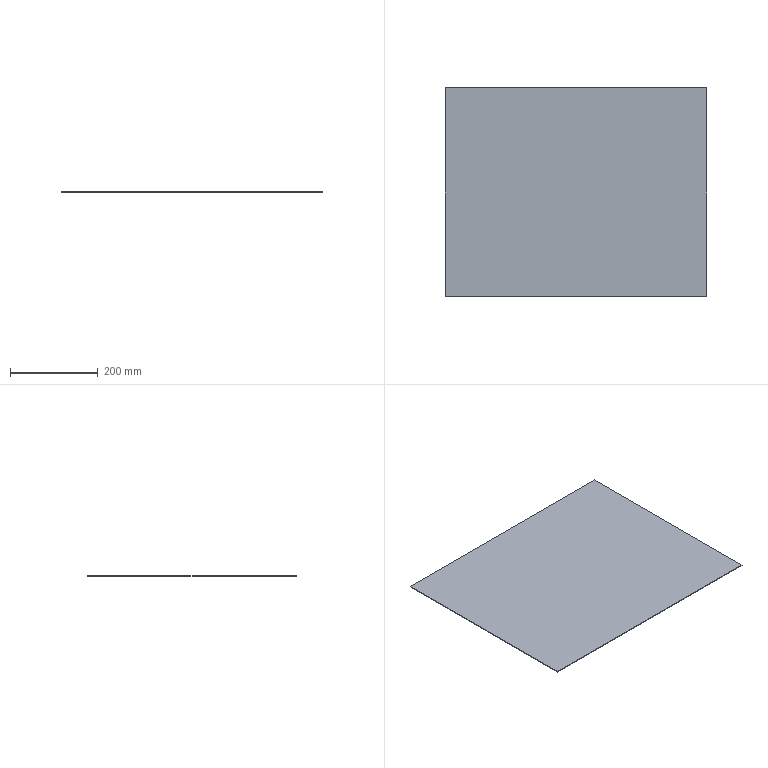Part | SolidWorks | features FlatPattern 1, SMBaseFlange 1, SheetMetal 1 | 1 solid | 6 faces | box 596 x 476 x 1.5 mm | volume 425544 mm3 | plane 6
STEP:
#1=CARTESIAN_POINT('',(298.,-238.,0.));
#2=VERTEX_POINT('',#1);
#3=CARTESIAN_POINT('',(298.,238.,0.));
#4=VERTEX_POINT('',#3);
#5=CARTESIAN_POINT('',(298.,-238.,0.));
#6=DIRECTION('',(0.,1.,0.));
#7=VECTOR('',#6,1000.);
#8=LINE('',#5,#7);
#9=EDGE_CURVE('',#2,#4,#8,.T.);
#10=ORIENTED_EDGE('',*,*,#9,.T.);
#11=CARTESIAN_POINT('',(298.,238.,1.5));
#12=VERTEX_POINT('',#11);
#13=CARTESIAN_POINT('',(298.,238.,1.5));
#14=DIRECTION('',(0.,0.,-1.));
#15=VECTOR('',#14,1000.);
#16=LINE('',#13,#15);
#17=EDGE_CURVE('',#12,#4,#16,.T.);
#18=ORIENTED_EDGE('',*,*,#17,.F.);
#19=CARTESIAN_POINT('',(298.,-238.,1.5));
#20=VERTEX_POINT('',#19);
#21=CARTESIAN_POINT('',(298.,-238.,1.5));
#22=DIRECTION('',(0.,1.,0.));
#23=VECTOR('',#22,1000.);
#24=LINE('',#21,#23);
#25=EDGE_CURVE('',#20,#12,#24,.T.);
#26=ORIENTED_EDGE('',*,*,#25,.F.);
#27=CARTESIAN_POINT('',(298.,-238.,1.5));
#28=DIRECTION('',(0.,0.,-1.));
#29=VECTOR('',#28,1000.);
#30=LINE('',#27,#29);
#31=EDGE_CURVE('',#20,#2,#30,.T.);
#32=ORIENTED_EDGE('',*,*,#31,.T.);
#33=EDGE_LOOP('',(#10,#18,#26,#32));
#34=FACE_OUTER_BOUND('',#33,.T.);
#35=CARTESIAN_POINT('',(298.,-238.,1.5));
#36=DIRECTION('',(-1.,0.,0.));
#37=DIRECTION('',(0.,0.,1.));
#38=AXIS2_PLACEMENT_3D('',#35,#36,#37);
#39=PLANE('',#38);
#40=ADVANCED_FACE('',(#34),#39,.F.);
#41=CARTESIAN_POINT('',(-298.,238.,0.));
#42=VERTEX_POINT('',#41);
#43=CARTESIAN_POINT('',(298.,238.,0.));
#44=DIRECTION('',(-1.,0.,0.));
#45=VECTOR('',#44,1000.);
#46=LINE('',#43,#45);
#47=EDGE_CURVE('',#4,#42,#46,.T.);
#48=ORIENTED_EDGE('',*,*,#47,.T.);
#49=CARTESIAN_POINT('',(-298.,238.,1.5));
#50=VERTEX_POINT('',#49);
#51=CARTESIAN_POINT('',(-298.,238.,1.5));
#52=DIRECTION('',(0.,0.,-1.));
#53=VECTOR('',#52,1000.);
#54=LINE('',#51,#53);
#55=EDGE_CURVE('',#50,#42,#54,.T.);
#56=ORIENTED_EDGE('',*,*,#55,.F.);
#57=CARTESIAN_POINT('',(298.,238.,1.5));
#58=DIRECTION('',(-1.,0.,0.));
#59=VECTOR('',#58,1000.);
#60=LINE('',#57,#59);
#61=EDGE_CURVE('',#12,#50,#60,.T.);
#62=ORIENTED_EDGE('',*,*,#61,.F.);
#63=ORIENTED_EDGE('',*,*,#17,.T.);
#64=EDGE_LOOP('',(#48,#56,#62,#63));
#65=FACE_OUTER_BOUND('',#64,.T.);
#66=CARTESIAN_POINT('',(298.,238.,1.5));
#67=DIRECTION('',(0.,-1.,0.));
#68=DIRECTION('',(0.,0.,-1.));
#69=AXIS2_PLACEMENT_3D('',#66,#67,#68);
#70=PLANE('',#69);
#71=ADVANCED_FACE('',(#65),#70,.F.);
#72=CARTESIAN_POINT('',(-298.,-238.,0.));
#73=VERTEX_POINT('',#72);
#74=CARTESIAN_POINT('',(-298.,-238.,0.));
#75=DIRECTION('',(0.,-1.,0.));
#76=VECTOR('',#75,1000.);
#77=LINE('',#74,#76);
#78=EDGE_CURVE('',#42,#73,#77,.T.);
#79=ORIENTED_EDGE('',*,*,#78,.T.);
#80=CARTESIAN_POINT('',(-298.,-238.,1.5));
#81=VERTEX_POINT('',#80);
#82=CARTESIAN_POINT('',(-298.,-238.,1.5));
#83=DIRECTION('',(0.,0.,-1.));
#84=VECTOR('',#83,1000.);
#85=LINE('',#82,#84);
#86=EDGE_CURVE('',#81,#73,#85,.T.);
#87=ORIENTED_EDGE('',*,*,#86,.F.);
#88=CARTESIAN_POINT('',(-298.,-238.,1.5));
#89=DIRECTION('',(0.,-1.,0.));
#90=VECTOR('',#89,1000.);
#91=LINE('',#88,#90);
#92=EDGE_CURVE('',#50,#81,#91,.T.);
#93=ORIENTED_EDGE('',*,*,#92,.F.);
#94=ORIENTED_EDGE('',*,*,#55,.T.);
#95=EDGE_LOOP('',(#79,#87,#93,#94));
#96=FACE_OUTER_BOUND('',#95,.T.);
#97=CARTESIAN_POINT('',(-298.,-238.,1.5));
#98=DIRECTION('',(1.,0.,0.));
#99=DIRECTION('',(0.,0.,-1.));
#100=AXIS2_PLACEMENT_3D('',#97,#98,#99);
#101=PLANE('',#100);
#102=ADVANCED_FACE('',(#96),#101,.F.);
#103=CARTESIAN_POINT('',(298.,-238.,0.));
#104=DIRECTION('',(1.,0.,0.));
#105=VECTOR('',#104,1000.);
#106=LINE('',#103,#105);
#107=EDGE_CURVE('',#73,#2,#106,.T.);
#108=ORIENTED_EDGE('',*,*,#107,.T.);
#109=ORIENTED_EDGE('',*,*,#31,.F.);
#110=CARTESIAN_POINT('',(298.,-238.,1.5));
#111=DIRECTION('',(1.,0.,0.));
#112=VECTOR('',#111,1000.);
#113=LINE('',#110,#112);
#114=EDGE_CURVE('',#81,#20,#113,.T.);
#115=ORIENTED_EDGE('',*,*,#114,.F.);
#116=ORIENTED_EDGE('',*,*,#86,.T.);
#117=EDGE_LOOP('',(#108,#109,#115,#116));
#118=FACE_OUTER_BOUND('',#117,.T.);
#119=CARTESIAN_POINT('',(298.,-238.,1.5));
#120=DIRECTION('',(0.,1.,0.));
#121=DIRECTION('',(0.,0.,1.));
#122=AXIS2_PLACEMENT_3D('',#119,#120,#121);
#123=PLANE('',#122);
#124=ADVANCED_FACE('',(#118),#123,.F.);
#125=ORIENTED_EDGE('',*,*,#25,.T.);
#126=ORIENTED_EDGE('',*,*,#61,.T.);
#127=ORIENTED_EDGE('',*,*,#92,.T.);
#128=ORIENTED_EDGE('',*,*,#114,.T.);
#129=EDGE_LOOP('',(#125,#126,#127,#128));
#130=FACE_OUTER_BOUND('',#129,.T.);
#131=CARTESIAN_POINT('',(0.,0.,1.5));
#132=DIRECTION('',(0.,0.,1.));
#133=DIRECTION('',(1.,0.,0.));
#134=AXIS2_PLACEMENT_3D('',#131,#132,#133);
#135=PLANE('',#134);
#136=ADVANCED_FACE('',(#130),#135,.T.);
#137=ORIENTED_EDGE('',*,*,#9,.F.);
#138=ORIENTED_EDGE('',*,*,#107,.F.);
#139=ORIENTED_EDGE('',*,*,#78,.F.);
#140=ORIENTED_EDGE('',*,*,#47,.F.);
#141=EDGE_LOOP('',(#137,#138,#139,#140));
#142=FACE_OUTER_BOUND('',#141,.T.);
#143=CARTESIAN_POINT('',(0.,0.,0.));
#144=DIRECTION('',(0.,0.,1.));
#145=DIRECTION('',(1.,0.,0.));
#146=AXIS2_PLACEMENT_3D('',#143,#144,#145);
#147=PLANE('',#146);
#148=ADVANCED_FACE('',(#142),#147,.F.);
#149=CLOSED_SHELL('',(#40,#71,#102,#124,#136,#148));
#150=MANIFOLD_SOLID_BREP('',#149);
#151=CARTESIAN_POINT('',(0.,0.,0.));
#152=DIRECTION('',(0.,0.,1.));
#153=DIRECTION('',(1.,0.,0.));
#154=AXIS2_PLACEMENT_3D('',#151,#152,#153);
#155=(LENGTH_UNIT()NAMED_UNIT(*)SI_UNIT(.MILLI.,.METRE.));
#156=UNCERTAINTY_MEASURE_WITH_UNIT(LENGTH_MEASURE(0.00001),#155,'','');
#157=(NAMED_UNIT(*)PLANE_ANGLE_UNIT()SI_UNIT($,.RADIAN.));
#158=(NAMED_UNIT(*)SI_UNIT($,.STERADIAN.)SOLID_ANGLE_UNIT());
#159=(GEOMETRIC_REPRESENTATION_CONTEXT(3)GLOBAL_UNCERTAINTY_ASSIGNED_CONTEXT((#156))GLOBAL_UNIT_ASSIGNED_CONTEXT((#155,#157,#158))REPRESENTATION_CONTEXT('',''));
#160=ADVANCED_BREP_SHAPE_REPRESENTATION('',(#150,#154),#159);